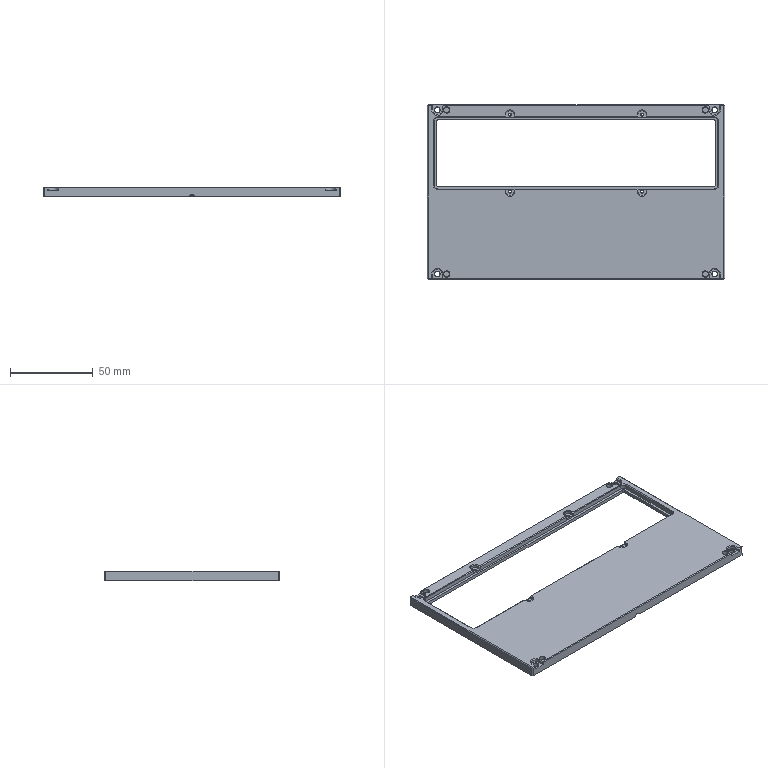Part | SolidWorks | features BaseBody 1 | 1 solid | 242 faces | box 180 x 105.4 x 6 mm | volume 51969 mm3 | plane 143 | cylinder 59 | cone 40 | commonest cylinder face diameters 2 x12 1.6 x8 3 x8 3.2 x8 3.5 x8 5 x8